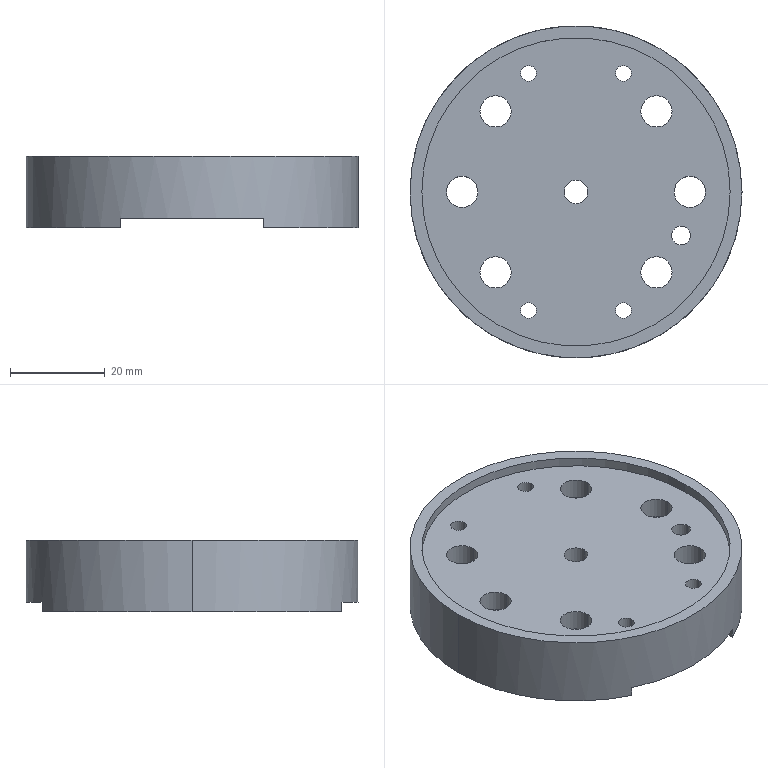Part | STEP file | C01 | 1 solid | 57 faces | box 70 x 70 x 15 mm | volume 40707 mm3 | cylinder 40 | plane 17 | commonest cylinder face diameters 6.6 x12 11 x12 3.3 x8 4 x2 5 x2 65 x2